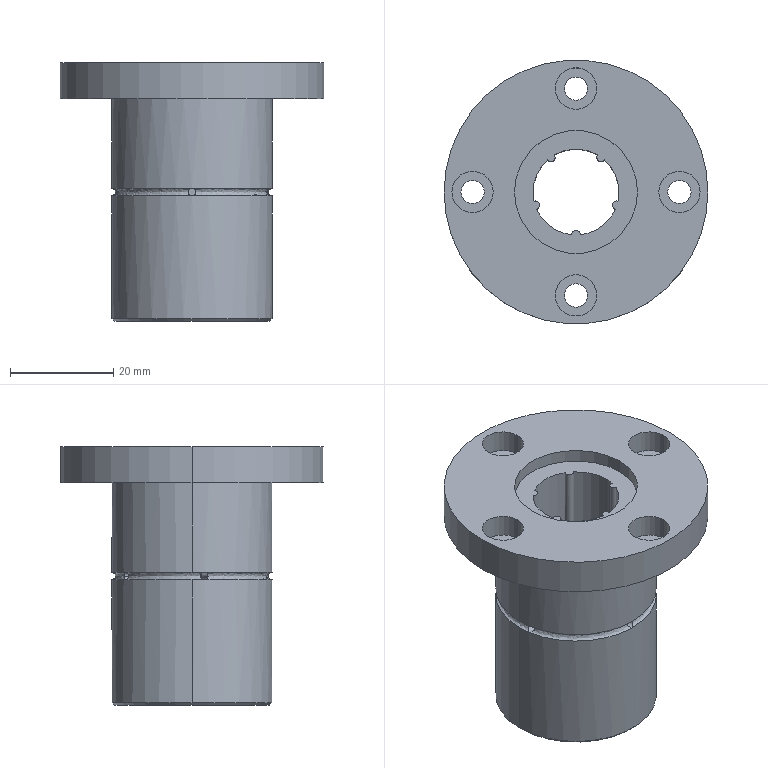Part | STEP file | 0229_Z_BSFM16-335-M8-NTW_2 | 1 solid | 67 faces | box 51 x 51 x 50 mm | volume 33822 mm3 | cylinder 50 | plane 9 | spline 6 | cone 2 | commonest cylinder face diameters 1.5 x10 1.66 x8 4.5 x8 8 x8 16.6 x6 23.8 x4